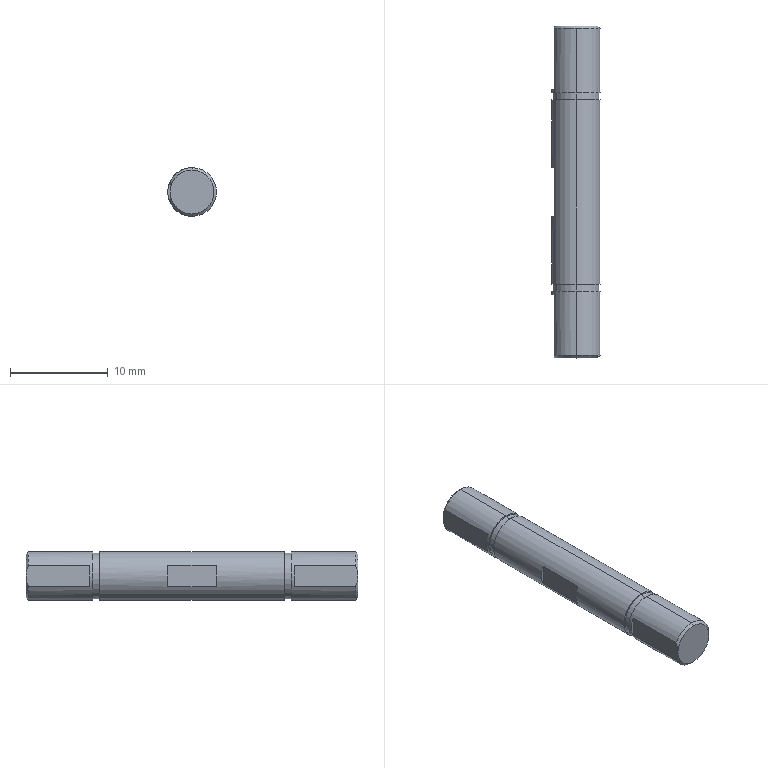Part | NX | features BREP 1 | 1 solid | 29 faces | box 5 x 34 x 5 mm | volume 656.944 mm3 | plane 13 | cylinder 10 | cone 6 | commonest cylinder face diameters 5 x6 4.7 x4
STEP:
#1=CARTESIAN_POINT('',(-2.25,-16.75,1.09));
#2=VERTEX_POINT('',#1);
#3=CARTESIAN_POINT('',(-2.25,-10.5,1.09));
#4=VERTEX_POINT('',#3);
#5=CARTESIAN_POINT('',(-2.25,-10.5,1.09));
#6=DIRECTION('',(0.,-1.,0.));
#7=VECTOR('',#6,1000.);
#8=LINE('',#5,#7);
#9=EDGE_CURVE('',#2,#4,#8,.F.);
#10=ORIENTED_EDGE('',*,*,#9,.T.);
#11=CARTESIAN_POINT('',(-2.25,-10.5,-1.09));
#12=VERTEX_POINT('',#11);
#13=CARTESIAN_POINT('',(-2.25,-10.5,1.09));
#14=DIRECTION('',(0.,0.,-1.));
#15=VECTOR('',#14,1000.);
#16=LINE('',#13,#15);
#17=EDGE_CURVE('',#4,#12,#16,.T.);
#18=ORIENTED_EDGE('',*,*,#17,.T.);
#19=CARTESIAN_POINT('',(-2.25,-16.75,-1.09));
#20=VERTEX_POINT('',#19);
#21=CARTESIAN_POINT('',(-2.25,-10.5,-1.09));
#22=DIRECTION('',(0.,-1.,0.));
#23=VECTOR('',#22,1000.);
#24=LINE('',#21,#23);
#25=EDGE_CURVE('',#20,#12,#24,.F.);
#26=ORIENTED_EDGE('',*,*,#25,.F.);
#27=CARTESIAN_POINT('',(-2.25,-17.,0.));
#28=VERTEX_POINT('',#27);
#29=CARTESIAN_POINT('',(-2.25,-16.75,-1.09));
#30=CARTESIAN_POINT('',(-2.25,-16.911,-0.7212));
#31=CARTESIAN_POINT('',(-2.25,-17.,-0.3659));
#32=CARTESIAN_POINT('',(-2.25,-17.,0.));
#33=B_SPLINE_CURVE_WITH_KNOTS('',3,(#29,#30,#31,#32),.UNSPECIFIED.,.F.,.F.,(4,4),(0.,1.),.UNSPECIFIED.);
#34=EDGE_CURVE('',#28,#20,#33,.F.);
#35=ORIENTED_EDGE('',*,*,#34,.F.);
#36=CARTESIAN_POINT('',(-2.25,-17.,0.));
#37=CARTESIAN_POINT('',(-2.25,-17.,0.3657));
#38=CARTESIAN_POINT('',(-2.25,-16.911,0.721));
#39=CARTESIAN_POINT('',(-2.25,-16.75,1.09));
#40=B_SPLINE_CURVE_WITH_KNOTS('',3,(#36,#37,#38,#39),.UNSPECIFIED.,.F.,.F.,(4,4),(0.,1.),.UNSPECIFIED.);
#41=EDGE_CURVE('',#2,#28,#40,.F.);
#42=ORIENTED_EDGE('',*,*,#41,.F.);
#43=EDGE_LOOP('',(#10,#18,#26,#35,#42));
#44=FACE_BOUND('',#43,.T.);
#45=CARTESIAN_POINT('',(-2.25,-10.5,1.09));
#46=DIRECTION('',(-1.,0.,0.));
#47=DIRECTION('',(0.,0.,1.));
#48=AXIS2_PLACEMENT_3D('',#45,#46,#47);
#49=PLANE('',#48);
#50=ADVANCED_FACE('',(#44),#49,.T.);
#51=ORIENTED_EDGE('',*,*,#17,.F.);
#52=CARTESIAN_POINT('',(0.,-10.5,0.));
#53=DIRECTION('',(0.,1.,0.));
#54=DIRECTION('',(0.,0.,1.));
#55=AXIS2_PLACEMENT_3D('',#52,#53,#54);
#56=CIRCLE('',#55,2.5);
#57=EDGE_CURVE('',#12,#4,#56,.T.);
#58=ORIENTED_EDGE('',*,*,#57,.F.);
#59=EDGE_LOOP('',(#51,#58));
#60=FACE_BOUND('',#59,.T.);
#61=CARTESIAN_POINT('',(0.,-10.5,0.));
#62=DIRECTION('',(0.,1.,0.));
#63=DIRECTION('',(0.,0.,-1.));
#64=AXIS2_PLACEMENT_3D('',#61,#62,#63);
#65=PLANE('',#64);
#66=ADVANCED_FACE('',(#60),#65,.F.);
#67=CARTESIAN_POINT('',(-2.25,16.75,1.09));
#68=VERTEX_POINT('',#67);
#69=CARTESIAN_POINT('',(-2.25,17.,0.));
#70=VERTEX_POINT('',#69);
#71=CARTESIAN_POINT('',(-2.25,16.75,1.09));
#72=CARTESIAN_POINT('',(-2.25,16.91,0.7218));
#73=CARTESIAN_POINT('',(-2.25,17.,0.3664));
#74=CARTESIAN_POINT('',(-2.25,17.,0.));
#75=B_SPLINE_CURVE_WITH_KNOTS('',3,(#71,#72,#73,#74),.UNSPECIFIED.,.F.,.F.,(4,4),(0.,1.),.UNSPECIFIED.);
#76=EDGE_CURVE('',#68,#70,#75,.T.);
#77=ORIENTED_EDGE('',*,*,#76,.T.);
#78=CARTESIAN_POINT('',(-2.25,16.75,-1.09));
#79=VERTEX_POINT('',#78);
#80=CARTESIAN_POINT('',(-2.25,17.,0.));
#81=CARTESIAN_POINT('',(-2.25,17.,-0.3652));
#82=CARTESIAN_POINT('',(-2.25,16.911,-0.7205));
#83=CARTESIAN_POINT('',(-2.25,16.75,-1.09));
#84=B_SPLINE_CURVE_WITH_KNOTS('',3,(#80,#81,#82,#83),.UNSPECIFIED.,.F.,.F.,(4,4),(0.,1.),.UNSPECIFIED.);
#85=EDGE_CURVE('',#70,#79,#84,.T.);
#86=ORIENTED_EDGE('',*,*,#85,.T.);
#87=CARTESIAN_POINT('',(-2.25,10.5,-1.09));
#88=VERTEX_POINT('',#87);
#89=CARTESIAN_POINT('',(-2.25,10.5,-1.09));
#90=DIRECTION('',(0.,1.,0.));
#91=VECTOR('',#90,1000.);
#92=LINE('',#89,#91);
#93=EDGE_CURVE('',#88,#79,#92,.T.);
#94=ORIENTED_EDGE('',*,*,#93,.F.);
#95=CARTESIAN_POINT('',(-2.25,10.5,1.09));
#96=VERTEX_POINT('',#95);
#97=CARTESIAN_POINT('',(-2.25,10.5,1.09));
#98=DIRECTION('',(0.,0.,-1.));
#99=VECTOR('',#98,1000.);
#100=LINE('',#97,#99);
#101=EDGE_CURVE('',#96,#88,#100,.T.);
#102=ORIENTED_EDGE('',*,*,#101,.F.);
#103=CARTESIAN_POINT('',(-2.25,10.5,1.09));
#104=DIRECTION('',(0.,1.,0.));
#105=VECTOR('',#104,1000.);
#106=LINE('',#103,#105);
#107=EDGE_CURVE('',#96,#68,#106,.T.);
#108=ORIENTED_EDGE('',*,*,#107,.T.);
#109=EDGE_LOOP('',(#77,#86,#94,#102,#108));
#110=FACE_BOUND('',#109,.T.);
#111=CARTESIAN_POINT('',(-2.25,10.5,1.09));
#112=DIRECTION('',(1.,0.,0.));
#113=DIRECTION('',(0.,0.,-1.));
#114=AXIS2_PLACEMENT_3D('',#111,#112,#113);
#115=PLANE('',#114);
#116=ADVANCED_FACE('',(#110),#115,.F.);
#117=ORIENTED_EDGE('',*,*,#101,.T.);
#118=CARTESIAN_POINT('',(0.,10.5,0.));
#119=DIRECTION('',(0.,-1.,0.));
#120=DIRECTION('',(0.,0.,-1.));
#121=AXIS2_PLACEMENT_3D('',#118,#119,#120);
#122=CIRCLE('',#121,2.5);
#123=EDGE_CURVE('',#96,#88,#122,.T.);
#124=ORIENTED_EDGE('',*,*,#123,.F.);
#125=EDGE_LOOP('',(#117,#124));
#126=FACE_BOUND('',#125,.T.);
#127=CARTESIAN_POINT('',(0.,10.5,0.));
#128=DIRECTION('',(0.,-1.,0.));
#129=DIRECTION('',(0.,0.,-1.));
#130=AXIS2_PLACEMENT_3D('',#127,#128,#129);
#131=PLANE('',#130);
#132=ADVANCED_FACE('',(#126),#131,.F.);
#133=CARTESIAN_POINT('',(-2.25,2.5,1.09));
#134=VERTEX_POINT('',#133);
#135=CARTESIAN_POINT('',(-2.25,2.5,-1.09));
#136=VERTEX_POINT('',#135);
#137=CARTESIAN_POINT('',(-2.25,2.5,1.09));
#138=DIRECTION('',(0.,0.,-1.));
#139=VECTOR('',#138,1000.);
#140=LINE('',#137,#139);
#141=EDGE_CURVE('',#134,#136,#140,.T.);
#142=ORIENTED_EDGE('',*,*,#141,.T.);
#143=CARTESIAN_POINT('',(-2.25,-2.5,-1.09));
#144=VERTEX_POINT('',#143);
#145=CARTESIAN_POINT('',(-2.25,-2.5,-1.09));
#146=DIRECTION('',(0.,1.,0.));
#147=VECTOR('',#146,1000.);
#148=LINE('',#145,#147);
#149=EDGE_CURVE('',#144,#136,#148,.T.);
#150=ORIENTED_EDGE('',*,*,#149,.F.);
#151=CARTESIAN_POINT('',(-2.25,-2.5,1.09));
#152=VERTEX_POINT('',#151);
#153=CARTESIAN_POINT('',(-2.25,-2.5,1.09));
#154=DIRECTION('',(0.,0.,-1.));
#155=VECTOR('',#154,1000.);
#156=LINE('',#153,#155);
#157=EDGE_CURVE('',#152,#144,#156,.T.);
#158=ORIENTED_EDGE('',*,*,#157,.F.);
#159=CARTESIAN_POINT('',(-2.25,-2.5,1.09));
#160=DIRECTION('',(0.,1.,0.));
#161=VECTOR('',#160,1000.);
#162=LINE('',#159,#161);
#163=EDGE_CURVE('',#152,#134,#162,.T.);
#164=ORIENTED_EDGE('',*,*,#163,.T.);
#165=EDGE_LOOP('',(#142,#150,#158,#164));
#166=FACE_BOUND('',#165,.T.);
#167=CARTESIAN_POINT('',(-2.25,-2.5,1.09));
#168=DIRECTION('',(1.,0.,0.));
#169=DIRECTION('',(0.,0.,-1.));
#170=AXIS2_PLACEMENT_3D('',#167,#168,#169);
#171=PLANE('',#170);
#172=ADVANCED_FACE('',(#166),#171,.F.);
#173=CARTESIAN_POINT('',(0.,2.5,0.));
#174=DIRECTION('',(0.,-1.,0.));
#175=DIRECTION('',(0.,0.,-1.));
#176=AXIS2_PLACEMENT_3D('',#173,#174,#175);
#177=CIRCLE('',#176,2.5);
#178=EDGE_CURVE('',#134,#136,#177,.T.);
#179=ORIENTED_EDGE('',*,*,#178,.T.);
#180=ORIENTED_EDGE('',*,*,#141,.F.);
#181=EDGE_LOOP('',(#179,#180));
#182=FACE_BOUND('',#181,.T.);
#183=CARTESIAN_POINT('',(0.,2.5,0.));
#184=DIRECTION('',(0.,-1.,0.));
#185=DIRECTION('',(0.,0.,-1.));
#186=AXIS2_PLACEMENT_3D('',#183,#184,#185);
#187=PLANE('',#186);
#188=ADVANCED_FACE('',(#182),#187,.T.);
#189=ORIENTED_EDGE('',*,*,#157,.T.);
#190=CARTESIAN_POINT('',(0.,-2.5,0.));
#191=DIRECTION('',(0.,-1.,0.));
#192=DIRECTION('',(0.,0.,-1.));
#193=AXIS2_PLACEMENT_3D('',#190,#191,#192);
#194=CIRCLE('',#193,2.5);
#195=EDGE_CURVE('',#152,#144,#194,.T.);
#196=ORIENTED_EDGE('',*,*,#195,.F.);
#197=EDGE_LOOP('',(#189,#196));
#198=FACE_BOUND('',#197,.T.);
#199=CARTESIAN_POINT('',(0.,-2.5,0.));
#200=DIRECTION('',(0.,-1.,0.));
#201=DIRECTION('',(0.,0.,-1.));
#202=AXIS2_PLACEMENT_3D('',#199,#200,#201);
#203=PLANE('',#202);
#204=ADVANCED_FACE('',(#198),#203,.F.);
#205=CARTESIAN_POINT('',(0.,17.,2.25));
#206=VERTEX_POINT('',#205);
#207=CARTESIAN_POINT('',(0.,16.75,2.5));
#208=VERTEX_POINT('',#207);
#209=CARTESIAN_POINT('',(0.,16.75,2.5));
#210=DIRECTION('',(0.,-0.7071,0.7071));
#211=VECTOR('',#210,1000.);
#212=LINE('',#209,#211);
#213=EDGE_CURVE('',#206,#208,#212,.T.);
#214=ORIENTED_EDGE('',*,*,#213,.F.);
#215=CARTESIAN_POINT('',(0.,17.,0.));
#216=DIRECTION('',(0.,1.,0.));
#217=DIRECTION('',(0.,0.,-1.));
#218=AXIS2_PLACEMENT_3D('',#215,#216,#217);
#219=CIRCLE('',#218,2.25);
#220=EDGE_CURVE('',#70,#206,#219,.T.);
#221=ORIENTED_EDGE('',*,*,#220,.F.);
#222=ORIENTED_EDGE('',*,*,#76,.F.);
#223=CARTESIAN_POINT('',(0.,16.75,0.));
#224=DIRECTION('',(0.,-1.,0.));
#225=DIRECTION('',(0.,0.,-1.));
#226=AXIS2_PLACEMENT_3D('',#223,#224,#225);
#227=CIRCLE('',#226,2.5);
#228=EDGE_CURVE('',#208,#68,#227,.T.);
#229=ORIENTED_EDGE('',*,*,#228,.F.);
#230=EDGE_LOOP('',(#214,#221,#222,#229));
#231=FACE_BOUND('',#230,.T.);
#232=CARTESIAN_POINT('',(0.,16.75,0.));
#233=DIRECTION('',(0.,-1.,0.));
#234=DIRECTION('',(0.,0.,-1.));
#235=AXIS2_PLACEMENT_3D('',#232,#233,#234);
#236=CONICAL_SURFACE('',#235,2.5,0.7854);
#237=ADVANCED_FACE('',(#231),#236,.T.);
#238=CARTESIAN_POINT('',(0.,-17.,-2.25));
#239=VERTEX_POINT('',#238);
#240=CARTESIAN_POINT('',(0.,-17.,0.));
#241=DIRECTION('',(0.,-1.,0.));
#242=DIRECTION('',(0.,0.,1.));
#243=AXIS2_PLACEMENT_3D('',#240,#241,#242);
#244=CIRCLE('',#243,2.25);
#245=EDGE_CURVE('',#28,#239,#244,.T.);
#246=ORIENTED_EDGE('',*,*,#245,.T.);
#247=CARTESIAN_POINT('',(0.,-17.,2.25));
#248=VERTEX_POINT('',#247);
#249=CARTESIAN_POINT('',(0.,-17.,0.));
#250=DIRECTION('',(0.,-1.,0.));
#251=DIRECTION('',(0.,0.,1.));
#252=AXIS2_PLACEMENT_3D('',#249,#250,#251);
#253=CIRCLE('',#252,2.25);
#254=EDGE_CURVE('',#239,#248,#253,.T.);
#255=ORIENTED_EDGE('',*,*,#254,.T.);
#256=CARTESIAN_POINT('',(0.,-17.,0.));
#257=DIRECTION('',(0.,-1.,0.));
#258=DIRECTION('',(0.,0.,1.));
#259=AXIS2_PLACEMENT_3D('',#256,#257,#258);
#260=CIRCLE('',#259,2.25);
#261=EDGE_CURVE('',#248,#28,#260,.T.);
#262=ORIENTED_EDGE('',*,*,#261,.T.);
#263=EDGE_LOOP('',(#246,#255,#262));
#264=FACE_BOUND('',#263,.T.);
#265=CARTESIAN_POINT('',(-2.5,-17.,0.));
#266=DIRECTION('',(0.,1.,0.));
#267=DIRECTION('',(0.,0.,1.));
#268=AXIS2_PLACEMENT_3D('',#265,#266,#267);
#269=PLANE('',#268);
#270=ADVANCED_FACE('',(#264),#269,.F.);
#271=CARTESIAN_POINT('',(0.,-10.15,-2.35));
#272=VERTEX_POINT('',#271);
#273=CARTESIAN_POINT('',(0.,-10.15,2.35));
#274=VERTEX_POINT('',#273);
#275=CARTESIAN_POINT('',(0.,-10.15,0.));
#276=DIRECTION('',(0.,-1.,0.));
#277=DIRECTION('',(0.,0.,-1.));
#278=AXIS2_PLACEMENT_3D('',#275,#276,#277);
#279=CIRCLE('',#278,2.35);
#280=EDGE_CURVE('',#272,#274,#279,.T.);
#281=ORIENTED_EDGE('',*,*,#280,.T.);
#282=CARTESIAN_POINT('',(0.,-10.15,0.));
#283=DIRECTION('',(0.,-1.,0.));
#284=DIRECTION('',(0.,0.,-1.));
#285=AXIS2_PLACEMENT_3D('',#282,#283,#284);
#286=CIRCLE('',#285,2.35);
#287=EDGE_CURVE('',#274,#272,#286,.T.);
#288=ORIENTED_EDGE('',*,*,#287,.T.);
#289=EDGE_LOOP('',(#281,#288));
#290=FACE_BOUND('',#289,.T.);
#291=CARTESIAN_POINT('',(0.,-10.15,-2.5));
#292=VERTEX_POINT('',#291);
#293=CARTESIAN_POINT('',(0.,-10.15,2.5));
#294=VERTEX_POINT('',#293);
#295=CARTESIAN_POINT('',(0.,-10.15,0.));
#296=DIRECTION('',(0.,-1.,0.));
#297=DIRECTION('',(0.,0.,-1.));
#298=AXIS2_PLACEMENT_3D('',#295,#296,#297);
#299=CIRCLE('',#298,2.5);
#300=EDGE_CURVE('',#292,#294,#299,.T.);
#301=ORIENTED_EDGE('',*,*,#300,.F.);
#302=CARTESIAN_POINT('',(0.,-10.15,0.));
#303=DIRECTION('',(0.,-1.,0.));
#304=DIRECTION('',(0.,0.,-1.));
#305=AXIS2_PLACEMENT_3D('',#302,#303,#304);
#306=CIRCLE('',#305,2.5);
#307=EDGE_CURVE('',#294,#292,#306,.T.);
#308=ORIENTED_EDGE('',*,*,#307,.F.);
#309=EDGE_LOOP('',(#301,#308));
#310=FACE_BOUND('',#309,.T.);
#311=CARTESIAN_POINT('',(-2.35,-10.15,0.));
#312=DIRECTION('',(0.,-1.,0.));
#313=DIRECTION('',(0.,0.,-1.));
#314=AXIS2_PLACEMENT_3D('',#311,#312,#313);
#315=PLANE('',#314);
#316=ADVANCED_FACE('',(#290,#310),#315,.F.);
#317=CARTESIAN_POINT('',(0.,-9.45,2.35));
#318=VERTEX_POINT('',#317);
#319=CARTESIAN_POINT('',(0.,-17.,2.35));
#320=DIRECTION('',(0.,-1.,0.));
#321=VECTOR('',#320,1000.);
#322=LINE('',#319,#321);
#323=EDGE_CURVE('',#318,#274,#322,.T.);
#324=ORIENTED_EDGE('',*,*,#323,.F.);
#325=CARTESIAN_POINT('',(0.,-9.45,-2.35));
#326=VERTEX_POINT('',#325);
#327=CARTESIAN_POINT('',(0.,-9.45,0.));
#328=DIRECTION('',(0.,-1.,0.));
#329=DIRECTION('',(0.,0.,-1.));
#330=AXIS2_PLACEMENT_3D('',#327,#328,#329);
#331=CIRCLE('',#330,2.35);
#332=EDGE_CURVE('',#318,#326,#331,.T.);
#333=ORIENTED_EDGE('',*,*,#332,.T.);
#334=CARTESIAN_POINT('',(0.,-17.,-2.35));
#335=DIRECTION('',(0.,-1.,0.));
#336=VECTOR('',#335,1000.);
#337=LINE('',#334,#336);
#338=EDGE_CURVE('',#326,#272,#337,.T.);
#339=ORIENTED_EDGE('',*,*,#338,.T.);
#340=ORIENTED_EDGE('',*,*,#287,.F.);
#341=EDGE_LOOP('',(#324,#333,#339,#340));
#342=FACE_BOUND('',#341,.T.);
#343=CARTESIAN_POINT('',(0.,-17.,0.));
#344=DIRECTION('',(0.,-1.,0.));
#345=DIRECTION('',(0.,0.,-1.));
#346=AXIS2_PLACEMENT_3D('',#343,#344,#345);
#347=CYLINDRICAL_SURFACE('',#346,2.35);
#348=ADVANCED_FACE('',(#342),#347,.T.);
#349=CARTESIAN_POINT('',(0.,-9.45,-2.5));
#350=VERTEX_POINT('',#349);
#351=CARTESIAN_POINT('',(0.,-9.45,2.5));
#352=VERTEX_POINT('',#351);
#353=CARTESIAN_POINT('',(0.,-9.45,0.));
#354=DIRECTION('',(0.,-1.,0.));
#355=DIRECTION('',(0.,0.,-1.));
#356=AXIS2_PLACEMENT_3D('',#353,#354,#355);
#357=CIRCLE('',#356,2.5);
#358=EDGE_CURVE('',#350,#352,#357,.T.);
#359=ORIENTED_EDGE('',*,*,#358,.T.);
#360=CARTESIAN_POINT('',(0.,-9.45,0.));
#361=DIRECTION('',(0.,-1.,0.));
#362=DIRECTION('',(0.,0.,-1.));
#363=AXIS2_PLACEMENT_3D('',#360,#361,#362);
#364=CIRCLE('',#363,2.5);
#365=EDGE_CURVE('',#352,#350,#364,.T.);
#366=ORIENTED_EDGE('',*,*,#365,.T.);
#367=EDGE_LOOP('',(#359,#366));
#368=FACE_BOUND('',#367,.T.);
#369=CARTESIAN_POINT('',(0.,-9.45,0.));
#370=DIRECTION('',(0.,-1.,0.));
#371=DIRECTION('',(0.,0.,-1.));
#372=AXIS2_PLACEMENT_3D('',#369,#370,#371);
#373=CIRCLE('',#372,2.35);
#374=EDGE_CURVE('',#326,#318,#373,.T.);
#375=ORIENTED_EDGE('',*,*,#374,.F.);
#376=ORIENTED_EDGE('',*,*,#332,.F.);
#377=EDGE_LOOP('',(#375,#376));
#378=FACE_BOUND('',#377,.T.);
#379=CARTESIAN_POINT('',(-2.5,-9.45,0.));
#380=DIRECTION('',(0.,1.,0.));
#381=DIRECTION('',(0.,0.,1.));
#382=AXIS2_PLACEMENT_3D('',#379,#380,#381);
#383=PLANE('',#382);
#384=ADVANCED_FACE('',(#368,#378),#383,.F.);
#385=ORIENTED_EDGE('',*,*,#163,.F.);
#386=ORIENTED_EDGE('',*,*,#195,.T.);
#387=ORIENTED_EDGE('',*,*,#149,.T.);
#388=ORIENTED_EDGE('',*,*,#178,.F.);
#389=EDGE_LOOP('',(#385,#386,#387,#388));
#390=FACE_BOUND('',#389,.T.);
#391=CARTESIAN_POINT('',(0.,9.45,2.5));
#392=VERTEX_POINT('',#391);
#393=CARTESIAN_POINT('',(0.,-17.,2.5));
#394=DIRECTION('',(0.,-1.,0.));
#395=VECTOR('',#394,1000.);
#396=LINE('',#393,#395);
#397=EDGE_CURVE('',#392,#352,#396,.T.);
#398=ORIENTED_EDGE('',*,*,#397,.F.);
#399=CARTESIAN_POINT('',(0.,9.45,-2.5));
#400=VERTEX_POINT('',#399);
#401=CARTESIAN_POINT('',(0.,9.45,0.));
#402=DIRECTION('',(0.,-1.,0.));
#403=DIRECTION('',(0.,0.,-1.));
#404=AXIS2_PLACEMENT_3D('',#401,#402,#403);
#405=CIRCLE('',#404,2.5);
#406=EDGE_CURVE('',#392,#400,#405,.T.);
#407=ORIENTED_EDGE('',*,*,#406,.T.);
#408=CARTESIAN_POINT('',(0.,-17.,-2.5));
#409=DIRECTION('',(0.,-1.,0.));
#410=VECTOR('',#409,1000.);
#411=LINE('',#408,#410);
#412=EDGE_CURVE('',#400,#350,#411,.T.);
#413=ORIENTED_EDGE('',*,*,#412,.T.);
#414=ORIENTED_EDGE('',*,*,#365,.F.);
#415=EDGE_LOOP('',(#398,#407,#413,#414));
#416=FACE_BOUND('',#415,.T.);
#417=CARTESIAN_POINT('',(0.,-17.,0.));
#418=DIRECTION('',(0.,-1.,0.));
#419=DIRECTION('',(0.,0.,-1.));
#420=AXIS2_PLACEMENT_3D('',#417,#418,#419);
#421=CYLINDRICAL_SURFACE('',#420,2.5);
#422=ADVANCED_FACE('',(#390,#416),#421,.T.);
#423=CARTESIAN_POINT('',(0.,9.45,-2.35));
#424=VERTEX_POINT('',#423);
#425=CARTESIAN_POINT('',(0.,9.45,2.35));
#426=VERTEX_POINT('',#425);
#427=CARTESIAN_POINT('',(0.,9.45,0.));
#428=DIRECTION('',(0.,-1.,0.));
#429=DIRECTION('',(0.,0.,-1.));
#430=AXIS2_PLACEMENT_3D('',#427,#428,#429);
#431=CIRCLE('',#430,2.35);
#432=EDGE_CURVE('',#424,#426,#431,.T.);
#433=ORIENTED_EDGE('',*,*,#432,.T.);
#434=CARTESIAN_POINT('',(0.,9.45,0.));
#435=DIRECTION('',(0.,-1.,0.));
#436=DIRECTION('',(0.,0.,-1.));
#437=AXIS2_PLACEMENT_3D('',#434,#435,#436);
#438=CIRCLE('',#437,2.35);
#439=EDGE_CURVE('',#426,#424,#438,.T.);
#440=ORIENTED_EDGE('',*,*,#439,.T.);
#441=EDGE_LOOP('',(#433,#440));
#442=FACE_BOUND('',#441,.T.);
#443=CARTESIAN_POINT('',(0.,9.45,0.));
#444=DIRECTION('',(0.,-1.,0.));
#445=DIRECTION('',(0.,0.,-1.));
#446=AXIS2_PLACEMENT_3D('',#443,#444,#445);
#447=CIRCLE('',#446,2.5);
#448=EDGE_CURVE('',#400,#392,#447,.T.);
#449=ORIENTED_EDGE('',*,*,#448,.F.);
#450=ORIENTED_EDGE('',*,*,#406,.F.);
#451=EDGE_LOOP('',(#449,#450));
#452=FACE_BOUND('',#451,.T.);
#453=CARTESIAN_POINT('',(-2.35,9.45,0.));
#454=DIRECTION('',(0.,-1.,0.));
#455=DIRECTION('',(0.,0.,-1.));
#456=AXIS2_PLACEMENT_3D('',#453,#454,#455);
#457=PLANE('',#456);
#458=ADVANCED_FACE('',(#442,#452),#457,.F.);
#459=CARTESIAN_POINT('',(0.,10.15,2.35));
#460=VERTEX_POINT('',#459);
#461=CARTESIAN_POINT('',(0.,-17.,2.35));
#462=DIRECTION('',(0.,-1.,0.));
#463=VECTOR('',#462,1000.);
#464=LINE('',#461,#463);
#465=EDGE_CURVE('',#460,#426,#464,.T.);
#466=ORIENTED_EDGE('',*,*,#465,.F.);
#467=CARTESIAN_POINT('',(0.,10.15,-2.35));
#468=VERTEX_POINT('',#467);
#469=CARTESIAN_POINT('',(0.,10.15,0.));
#470=DIRECTION('',(0.,-1.,0.));
#471=DIRECTION('',(0.,0.,-1.));
#472=AXIS2_PLACEMENT_3D('',#469,#470,#471);
#473=CIRCLE('',#472,2.35);
#474=EDGE_CURVE('',#460,#468,#473,.T.);
#475=ORIENTED_EDGE('',*,*,#474,.T.);
#476=CARTESIAN_POINT('',(0.,-17.,-2.35));
#477=DIRECTION('',(0.,-1.,0.));
#478=VECTOR('',#477,1000.);
#479=LINE('',#476,#478);
#480=EDGE_CURVE('',#468,#424,#479,.T.);
#481=ORIENTED_EDGE('',*,*,#480,.T.);
#482=ORIENTED_EDGE('',*,*,#439,.F.);
#483=EDGE_LOOP('',(#466,#475,#481,#482));
#484=FACE_BOUND('',#483,.T.);
#485=CARTESIAN_POINT('',(0.,-17.,0.));
#486=DIRECTION('',(0.,-1.,0.));
#487=DIRECTION('',(0.,0.,-1.));
#488=AXIS2_PLACEMENT_3D('',#485,#486,#487);
#489=CYLINDRICAL_SURFACE('',#488,2.35);
#490=ADVANCED_FACE('',(#484),#489,.T.);
#491=CARTESIAN_POINT('',(0.,10.15,-2.5));
#492=VERTEX_POINT('',#491);
#493=CARTESIAN_POINT('',(0.,10.15,2.5));
#494=VERTEX_POINT('',#493);
#495=CARTESIAN_POINT('',(0.,10.15,0.));
#496=DIRECTION('',(0.,-1.,0.));
#497=DIRECTION('',(0.,0.,-1.));
#498=AXIS2_PLACEMENT_3D('',#495,#496,#497);
#499=CIRCLE('',#498,2.5);
#500=EDGE_CURVE('',#492,#494,#499,.T.);
#501=ORIENTED_EDGE('',*,*,#500,.T.);
#502=CARTESIAN_POINT('',(0.,10.15,0.));
#503=DIRECTION('',(0.,-1.,0.));
#504=DIRECTION('',(0.,0.,-1.));
#505=AXIS2_PLACEMENT_3D('',#502,#503,#504);
#506=CIRCLE('',#505,2.5);
#507=EDGE_CURVE('',#494,#492,#506,.T.);
#508=ORIENTED_EDGE('',*,*,#507,.T.);
#509=EDGE_LOOP('',(#501,#508));
#510=FACE_BOUND('',#509,.T.);
#511=CARTESIAN_POINT('',(0.,10.15,0.));
#512=DIRECTION('',(0.,-1.,0.));
#513=DIRECTION('',(0.,0.,-1.));
#514=AXIS2_PLACEMENT_3D('',#511,#512,#513);
#515=CIRCLE('',#514,2.35);
#516=EDGE_CURVE('',#468,#460,#515,.T.);
#517=ORIENTED_EDGE('',*,*,#516,.F.);
#518=ORIENTED_EDGE('',*,*,#474,.F.);
#519=EDGE_LOOP('',(#517,#518));
#520=FACE_BOUND('',#519,.T.);
#521=CARTESIAN_POINT('',(-2.5,10.15,0.));
#522=DIRECTION('',(0.,1.,0.));
#523=DIRECTION('',(0.,0.,1.));
#524=AXIS2_PLACEMENT_3D('',#521,#522,#523);
#525=PLANE('',#524);
#526=ADVANCED_FACE('',(#510,#520),#525,.F.);
#527=CARTESIAN_POINT('',(0.,-17.,2.5));
#528=DIRECTION('',(0.,-1.,0.));
#529=VECTOR('',#528,1000.);
#530=LINE('',#527,#529);
#531=EDGE_CURVE('',#208,#494,#530,.T.);
#532=ORIENTED_EDGE('',*,*,#531,.F.);
#533=ORIENTED_EDGE('',*,*,#228,.T.);
#534=ORIENTED_EDGE('',*,*,#107,.F.);
#535=ORIENTED_EDGE('',*,*,#123,.T.);
#536=ORIENTED_EDGE('',*,*,#93,.T.);
#537=CARTESIAN_POINT('',(0.,16.75,-2.5));
#538=VERTEX_POINT('',#537);
#539=CARTESIAN_POINT('',(0.,16.75,0.));
#540=DIRECTION('',(0.,-1.,0.));
#541=DIRECTION('',(0.,0.,-1.));
#542=AXIS2_PLACEMENT_3D('',#539,#540,#541);
#543=CIRCLE('',#542,2.5);
#544=EDGE_CURVE('',#79,#538,#543,.T.);
#545=ORIENTED_EDGE('',*,*,#544,.T.);
#546=CARTESIAN_POINT('',(0.,-17.,-2.5));
#547=DIRECTION('',(0.,-1.,0.));
#548=VECTOR('',#547,1000.);
#549=LINE('',#546,#548);
#550=EDGE_CURVE('',#538,#492,#549,.T.);
#551=ORIENTED_EDGE('',*,*,#550,.T.);
#552=ORIENTED_EDGE('',*,*,#507,.F.);
#553=EDGE_LOOP('',(#532,#533,#534,#535,#536,#545,#551,#552));
#554=FACE_BOUND('',#553,.T.);
#555=CARTESIAN_POINT('',(0.,-17.,0.));
#556=DIRECTION('',(0.,-1.,0.));
#557=DIRECTION('',(0.,0.,-1.));
#558=AXIS2_PLACEMENT_3D('',#555,#556,#557);
#559=CYLINDRICAL_SURFACE('',#558,2.5);
#560=ADVANCED_FACE('',(#554),#559,.T.);
#561=ORIENTED_EDGE('',*,*,#220,.T.);
#562=CARTESIAN_POINT('',(0.,17.,-2.25));
#563=VERTEX_POINT('',#562);
#564=CARTESIAN_POINT('',(0.,17.,0.));
#565=DIRECTION('',(0.,1.,0.));
#566=DIRECTION('',(0.,0.,-1.));
#567=AXIS2_PLACEMENT_3D('',#564,#565,#566);
#568=CIRCLE('',#567,2.25);
#569=EDGE_CURVE('',#206,#563,#568,.T.);
#570=ORIENTED_EDGE('',*,*,#569,.T.);
#571=CARTESIAN_POINT('',(0.,17.,0.));
#572=DIRECTION('',(0.,1.,0.));
#573=DIRECTION('',(0.,0.,-1.));
#574=AXIS2_PLACEMENT_3D('',#571,#572,#573);
#575=CIRCLE('',#574,2.25);
#576=EDGE_CURVE('',#563,#70,#575,.T.);
#577=ORIENTED_EDGE('',*,*,#576,.T.);
#578=EDGE_LOOP('',(#561,#570,#577));
#579=FACE_BOUND('',#578,.T.);
#580=CARTESIAN_POINT('',(0.,17.,0.));
#581=DIRECTION('',(0.,-1.,0.));
#582=DIRECTION('',(0.,0.,-1.));
#583=AXIS2_PLACEMENT_3D('',#580,#581,#582);
#584=PLANE('',#583);
#585=ADVANCED_FACE('',(#579),#584,.F.);
#586=CARTESIAN_POINT('',(0.,-16.75,-2.5));
#587=VERTEX_POINT('',#586);
#588=CARTESIAN_POINT('',(0.,-17.,-2.25));
#589=DIRECTION('',(0.,0.7071,-0.7071));
#590=VECTOR('',#589,1000.);
#591=LINE('',#588,#590);
#592=EDGE_CURVE('',#239,#587,#591,.T.);
#593=ORIENTED_EDGE('',*,*,#592,.F.);
#594=ORIENTED_EDGE('',*,*,#245,.F.);
#595=ORIENTED_EDGE('',*,*,#34,.T.);
#596=CARTESIAN_POINT('',(0.,-16.75,0.));
#597=DIRECTION('',(0.,1.,0.));
#598=DIRECTION('',(0.,0.,1.));
#599=AXIS2_PLACEMENT_3D('',#596,#597,#598);
#600=CIRCLE('',#599,2.5);
#601=EDGE_CURVE('',#587,#20,#600,.T.);
#602=ORIENTED_EDGE('',*,*,#601,.F.);
#603=EDGE_LOOP('',(#593,#594,#595,#602));
#604=FACE_BOUND('',#603,.T.);
#605=CARTESIAN_POINT('',(0.,-17.,0.));
#606=DIRECTION('',(0.,1.,0.));
#607=DIRECTION('',(0.,0.,1.));
#608=AXIS2_PLACEMENT_3D('',#605,#606,#607);
#609=CONICAL_SURFACE('',#608,2.25,0.7854);
#610=ADVANCED_FACE('',(#604),#609,.T.);
#611=CARTESIAN_POINT('',(0.,-16.75,2.5));
#612=VERTEX_POINT('',#611);
#613=CARTESIAN_POINT('',(0.,-17.,2.5));
#614=DIRECTION('',(0.,-1.,0.));
#615=VECTOR('',#614,1000.);
#616=LINE('',#613,#615);
#617=EDGE_CURVE('',#294,#612,#616,.T.);
#618=ORIENTED_EDGE('',*,*,#617,.F.);
#619=ORIENTED_EDGE('',*,*,#307,.T.);
#620=CARTESIAN_POINT('',(0.,-17.,-2.5));
#621=DIRECTION('',(0.,-1.,0.));
#622=VECTOR('',#621,1000.);
#623=LINE('',#620,#622);
#624=EDGE_CURVE('',#292,#587,#623,.T.);
#625=ORIENTED_EDGE('',*,*,#624,.T.);
#626=ORIENTED_EDGE('',*,*,#601,.T.);
#627=ORIENTED_EDGE('',*,*,#25,.T.);
#628=ORIENTED_EDGE('',*,*,#57,.T.);
#629=ORIENTED_EDGE('',*,*,#9,.F.);
#630=CARTESIAN_POINT('',(0.,-16.75,0.));
#631=DIRECTION('',(0.,1.,0.));
#632=DIRECTION('',(0.,0.,1.));
#633=AXIS2_PLACEMENT_3D('',#630,#631,#632);
#634=CIRCLE('',#633,2.5);
#635=EDGE_CURVE('',#2,#612,#634,.T.);
#636=ORIENTED_EDGE('',*,*,#635,.T.);
#637=EDGE_LOOP('',(#618,#619,#625,#626,#627,#628,#629,#636));
#638=FACE_BOUND('',#637,.T.);
#639=CARTESIAN_POINT('',(0.,-17.,0.));
#640=DIRECTION('',(0.,-1.,0.));
#641=DIRECTION('',(0.,0.,-1.));
#642=AXIS2_PLACEMENT_3D('',#639,#640,#641);
#643=CYLINDRICAL_SURFACE('',#642,2.5);
#644=ADVANCED_FACE('',(#638),#643,.T.);
#645=ORIENTED_EDGE('',*,*,#300,.T.);
#646=ORIENTED_EDGE('',*,*,#617,.T.);
#647=CARTESIAN_POINT('',(0.,-16.75,0.));
#648=DIRECTION('',(0.,1.,0.));
#649=DIRECTION('',(0.,0.,1.));
#650=AXIS2_PLACEMENT_3D('',#647,#648,#649);
#651=CIRCLE('',#650,2.5);
#652=EDGE_CURVE('',#612,#587,#651,.T.);
#653=ORIENTED_EDGE('',*,*,#652,.T.);
#654=ORIENTED_EDGE('',*,*,#624,.F.);
#655=EDGE_LOOP('',(#645,#646,#653,#654));
#656=FACE_BOUND('',#655,.T.);
#657=CARTESIAN_POINT('',(0.,-17.,0.));
#658=DIRECTION('',(0.,-1.,0.));
#659=DIRECTION('',(0.,0.,-1.));
#660=AXIS2_PLACEMENT_3D('',#657,#658,#659);
#661=CYLINDRICAL_SURFACE('',#660,2.5);
#662=ADVANCED_FACE('',(#656),#661,.T.);
#663=ORIENTED_EDGE('',*,*,#261,.F.);
#664=CARTESIAN_POINT('',(0.,-17.,2.25));
#665=DIRECTION('',(0.,0.7071,0.7071));
#666=VECTOR('',#665,1000.);
#667=LINE('',#664,#666);
#668=EDGE_CURVE('',#248,#612,#667,.T.);
#669=ORIENTED_EDGE('',*,*,#668,.T.);
#670=ORIENTED_EDGE('',*,*,#635,.F.);
#671=ORIENTED_EDGE('',*,*,#41,.T.);
#672=EDGE_LOOP('',(#663,#669,#670,#671));
#673=FACE_BOUND('',#672,.T.);
#674=CARTESIAN_POINT('',(0.,-17.,0.));
#675=DIRECTION('',(0.,1.,0.));
#676=DIRECTION('',(0.,0.,1.));
#677=AXIS2_PLACEMENT_3D('',#674,#675,#676);
#678=CONICAL_SURFACE('',#677,2.25,0.7854);
#679=ADVANCED_FACE('',(#673),#678,.T.);
#680=ORIENTED_EDGE('',*,*,#254,.F.);
#681=ORIENTED_EDGE('',*,*,#592,.T.);
#682=ORIENTED_EDGE('',*,*,#652,.F.);
#683=ORIENTED_EDGE('',*,*,#668,.F.);
#684=EDGE_LOOP('',(#680,#681,#682,#683));
#685=FACE_BOUND('',#684,.T.);
#686=CARTESIAN_POINT('',(0.,-17.,0.));
#687=DIRECTION('',(0.,1.,0.));
#688=DIRECTION('',(0.,0.,1.));
#689=AXIS2_PLACEMENT_3D('',#686,#687,#688);
#690=CONICAL_SURFACE('',#689,2.25,0.7854);
#691=ADVANCED_FACE('',(#685),#690,.T.);
#692=CARTESIAN_POINT('',(0.,16.75,0.));
#693=DIRECTION('',(0.,-1.,0.));
#694=DIRECTION('',(0.,0.,-1.));
#695=AXIS2_PLACEMENT_3D('',#692,#693,#694);
#696=CIRCLE('',#695,2.5);
#697=EDGE_CURVE('',#538,#208,#696,.T.);
#698=ORIENTED_EDGE('',*,*,#697,.T.);
#699=ORIENTED_EDGE('',*,*,#531,.T.);
#700=ORIENTED_EDGE('',*,*,#500,.F.);
#701=ORIENTED_EDGE('',*,*,#550,.F.);
#702=EDGE_LOOP('',(#698,#699,#700,#701));
#703=FACE_BOUND('',#702,.T.);
#704=CARTESIAN_POINT('',(0.,-17.,0.));
#705=DIRECTION('',(0.,-1.,0.));
#706=DIRECTION('',(0.,0.,-1.));
#707=AXIS2_PLACEMENT_3D('',#704,#705,#706);
#708=CYLINDRICAL_SURFACE('',#707,2.5);
#709=ADVANCED_FACE('',(#703),#708,.T.);
#710=ORIENTED_EDGE('',*,*,#516,.T.);
#711=ORIENTED_EDGE('',*,*,#465,.T.);
#712=ORIENTED_EDGE('',*,*,#432,.F.);
#713=ORIENTED_EDGE('',*,*,#480,.F.);
#714=EDGE_LOOP('',(#710,#711,#712,#713));
#715=FACE_BOUND('',#714,.T.);
#716=CARTESIAN_POINT('',(0.,-17.,0.));
#717=DIRECTION('',(0.,-1.,0.));
#718=DIRECTION('',(0.,0.,-1.));
#719=AXIS2_PLACEMENT_3D('',#716,#717,#718);
#720=CYLINDRICAL_SURFACE('',#719,2.35);
#721=ADVANCED_FACE('',(#715),#720,.T.);
#722=ORIENTED_EDGE('',*,*,#448,.T.);
#723=ORIENTED_EDGE('',*,*,#397,.T.);
#724=ORIENTED_EDGE('',*,*,#358,.F.);
#725=ORIENTED_EDGE('',*,*,#412,.F.);
#726=EDGE_LOOP('',(#722,#723,#724,#725));
#727=FACE_BOUND('',#726,.T.);
#728=CARTESIAN_POINT('',(0.,-17.,0.));
#729=DIRECTION('',(0.,-1.,0.));
#730=DIRECTION('',(0.,0.,-1.));
#731=AXIS2_PLACEMENT_3D('',#728,#729,#730);
#732=CYLINDRICAL_SURFACE('',#731,2.5);
#733=ADVANCED_FACE('',(#727),#732,.T.);
#734=ORIENTED_EDGE('',*,*,#374,.T.);
#735=ORIENTED_EDGE('',*,*,#323,.T.);
#736=ORIENTED_EDGE('',*,*,#280,.F.);
#737=ORIENTED_EDGE('',*,*,#338,.F.);
#738=EDGE_LOOP('',(#734,#735,#736,#737));
#739=FACE_BOUND('',#738,.T.);
#740=CARTESIAN_POINT('',(0.,-17.,0.));
#741=DIRECTION('',(0.,-1.,0.));
#742=DIRECTION('',(0.,0.,-1.));
#743=AXIS2_PLACEMENT_3D('',#740,#741,#742);
#744=CYLINDRICAL_SURFACE('',#743,2.35);
#745=ADVANCED_FACE('',(#739),#744,.T.);
#746=ORIENTED_EDGE('',*,*,#576,.F.);
#747=CARTESIAN_POINT('',(0.,16.75,-2.5));
#748=DIRECTION('',(0.,-0.7071,-0.7071));
#749=VECTOR('',#748,1000.);
#750=LINE('',#747,#749);
#751=EDGE_CURVE('',#563,#538,#750,.T.);
#752=ORIENTED_EDGE('',*,*,#751,.T.);
#753=ORIENTED_EDGE('',*,*,#544,.F.);
#754=ORIENTED_EDGE('',*,*,#85,.F.);
#755=EDGE_LOOP('',(#746,#752,#753,#754));
#756=FACE_BOUND('',#755,.T.);
#757=CARTESIAN_POINT('',(0.,16.75,0.));
#758=DIRECTION('',(0.,-1.,0.));
#759=DIRECTION('',(0.,0.,-1.));
#760=AXIS2_PLACEMENT_3D('',#757,#758,#759);
#761=CONICAL_SURFACE('',#760,2.5,0.7854);
#762=ADVANCED_FACE('',(#756),#761,.T.);
#763=ORIENTED_EDGE('',*,*,#569,.F.);
#764=ORIENTED_EDGE('',*,*,#213,.T.);
#765=ORIENTED_EDGE('',*,*,#697,.F.);
#766=ORIENTED_EDGE('',*,*,#751,.F.);
#767=EDGE_LOOP('',(#763,#764,#765,#766));
#768=FACE_BOUND('',#767,.T.);
#769=CARTESIAN_POINT('',(0.,16.75,0.));
#770=DIRECTION('',(0.,-1.,0.));
#771=DIRECTION('',(0.,0.,-1.));
#772=AXIS2_PLACEMENT_3D('',#769,#770,#771);
#773=CONICAL_SURFACE('',#772,2.5,0.7854);
#774=ADVANCED_FACE('',(#768),#773,.T.);
#775=CLOSED_SHELL('',(#50,#66,#116,#132,#172,#188,#204,#237,#270,#316,#348,#384,#422,#458,#490,#526,#560,#585,#610,#644,#662,#679,#691,#709,#721,#733,#745,#762,#774));
#776=MANIFOLD_SOLID_BREP('',#775);
#777=(LENGTH_UNIT()NAMED_UNIT(*)SI_UNIT(.MILLI.,.METRE.));
#778=UNCERTAINTY_MEASURE_WITH_UNIT(LENGTH_MEASURE(0.0508),#777,'','');
#779=(NAMED_UNIT(*)PLANE_ANGLE_UNIT()SI_UNIT($,.RADIAN.));
#780=(NAMED_UNIT(*)SI_UNIT($,.STERADIAN.)SOLID_ANGLE_UNIT());
#781=(GEOMETRIC_REPRESENTATION_CONTEXT(3)GLOBAL_UNCERTAINTY_ASSIGNED_CONTEXT((#778))GLOBAL_UNIT_ASSIGNED_CONTEXT((#777,#779,#780))REPRESENTATION_CONTEXT('',''));
#782=ADVANCED_BREP_SHAPE_REPRESENTATION('',(#776),#781);